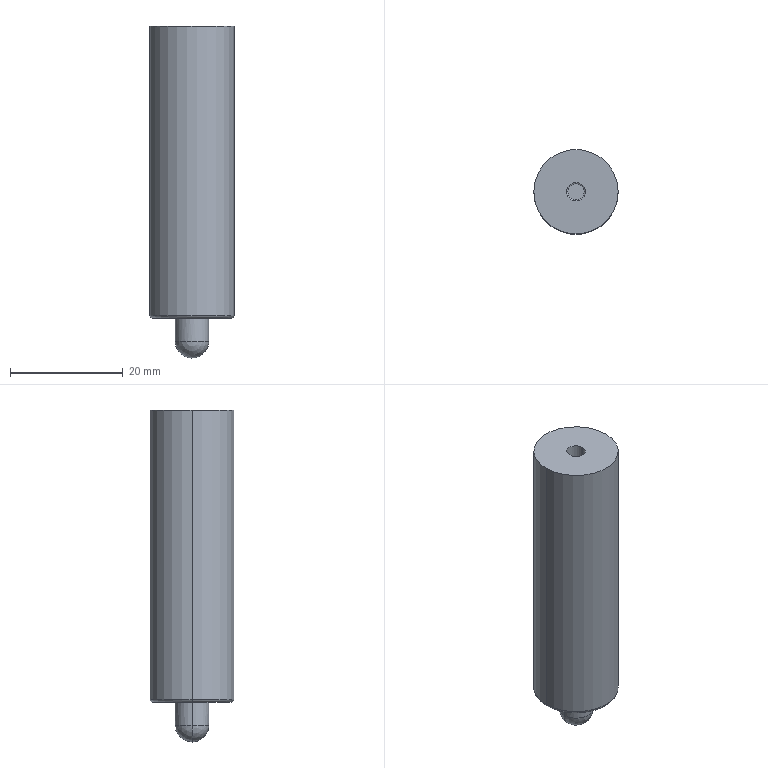Part | SolidWorks | features BaseBody 1, HoleWzd 1, MoveFace 1 | 1 solid | 18 faces | box 15 x 15 x 59 mm | volume 9190 mm3 | cylinder 8 | torus 3 | plane 3 | cone 2 | sphere 2 | commonest cylinder face diameters 2.9 x2 3.3 x2 6 x2 15 x2
STEP:
#1=CARTESIAN_POINT('',(-699.78,615.797,484.382));
#2=VERTEX_POINT('',#1);
#3=CARTESIAN_POINT('',(-696.48,615.797,484.382));
#4=VERTEX_POINT('',#3);
#5=CARTESIAN_POINT('',(-698.13,615.797,484.382));
#6=DIRECTION('',(0.,0.,1.));
#7=DIRECTION('',(1.,0.,0.));
#8=AXIS2_PLACEMENT_3D('',#5,#6,#7);
#9=CIRCLE('',#8,1.65);
#10=EDGE_CURVE('',#2,#4,#9,.T.);
#11=ORIENTED_EDGE('',*,*,#10,.F.);
#12=CARTESIAN_POINT('',(-699.78,615.797,494.482));
#13=VERTEX_POINT('',#12);
#14=CARTESIAN_POINT('',(-699.78,615.797,494.482));
#15=DIRECTION('',(0.,0.,1.));
#16=VECTOR('',#15,1000.);
#17=LINE('',#14,#16);
#18=EDGE_CURVE('',#2,#13,#17,.T.);
#19=ORIENTED_EDGE('',*,*,#18,.T.);
#20=CARTESIAN_POINT('',(-696.48,615.797,494.482));
#21=VERTEX_POINT('',#20);
#22=CARTESIAN_POINT('',(-698.13,615.797,494.482));
#23=DIRECTION('',(0.,0.,1.));
#24=DIRECTION('',(1.,0.,0.));
#25=AXIS2_PLACEMENT_3D('',#22,#23,#24);
#26=CIRCLE('',#25,1.65);
#27=EDGE_CURVE('',#13,#21,#26,.T.);
#28=ORIENTED_EDGE('',*,*,#27,.T.);
#29=CARTESIAN_POINT('',(-696.48,615.797,494.482));
#30=DIRECTION('',(0.,0.,1.));
#31=VECTOR('',#30,1000.);
#32=LINE('',#29,#31);
#33=EDGE_CURVE('',#4,#21,#32,.T.);
#34=ORIENTED_EDGE('',*,*,#33,.F.);
#35=EDGE_LOOP('',(#11,#19,#28,#34));
#36=FACE_OUTER_BOUND('',#35,.T.);
#37=CARTESIAN_POINT('',(-698.13,615.797,494.482));
#38=DIRECTION('',(0.,0.,1.));
#39=DIRECTION('',(1.,0.,0.));
#40=AXIS2_PLACEMENT_3D('',#37,#38,#39);
#41=CYLINDRICAL_SURFACE('',#40,1.65);
#42=ADVANCED_FACE('',(#36),#41,.F.);
#43=CARTESIAN_POINT('',(-699.58,615.797,484.262));
#44=VERTEX_POINT('',#43);
#45=CARTESIAN_POINT('',(-696.68,615.797,484.262));
#46=VERTEX_POINT('',#45);
#47=CARTESIAN_POINT('',(-698.13,615.797,484.262));
#48=DIRECTION('',(0.,0.,1.));
#49=DIRECTION('',(1.,0.,0.));
#50=AXIS2_PLACEMENT_3D('',#47,#48,#49);
#51=CIRCLE('',#50,1.45);
#52=EDGE_CURVE('',#44,#46,#51,.T.);
#53=ORIENTED_EDGE('',*,*,#52,.F.);
#54=CARTESIAN_POINT('',(-699.78,615.797,484.382));
#55=DIRECTION('',(-0.8572,0.,0.515));
#56=VECTOR('',#55,1000.);
#57=LINE('',#54,#56);
#58=EDGE_CURVE('',#44,#2,#57,.T.);
#59=ORIENTED_EDGE('',*,*,#58,.T.);
#60=ORIENTED_EDGE('',*,*,#10,.T.);
#61=CARTESIAN_POINT('',(-696.48,615.797,484.382));
#62=DIRECTION('',(0.8572,0.,0.515));
#63=VECTOR('',#62,1000.);
#64=LINE('',#61,#63);
#65=EDGE_CURVE('',#46,#4,#64,.T.);
#66=ORIENTED_EDGE('',*,*,#65,.F.);
#67=EDGE_LOOP('',(#53,#59,#60,#66));
#68=FACE_OUTER_BOUND('',#67,.T.);
#69=CARTESIAN_POINT('',(-698.13,615.797,484.382));
#70=DIRECTION('',(0.,0.,1.));
#71=DIRECTION('',(1.,0.,0.));
#72=AXIS2_PLACEMENT_3D('',#69,#70,#71);
#73=CONICAL_SURFACE('',#72,1.65,1.03);
#74=ADVANCED_FACE('',(#68),#73,.F.);
#75=CARTESIAN_POINT('',(-690.63,615.894,443.08));
#76=VERTEX_POINT('',#75);
#77=CARTESIAN_POINT('',(-705.63,615.797,443.08));
#78=VERTEX_POINT('',#77);
#79=CARTESIAN_POINT('',(-698.13,615.797,443.08));
#80=DIRECTION('',(0.,0.,1.));
#81=DIRECTION('',(0.9999,0.01286,0.));
#82=AXIS2_PLACEMENT_3D('',#79,#80,#81);
#83=CIRCLE('',#82,7.5);
#84=EDGE_CURVE('',#76,#78,#83,.T.);
#85=ORIENTED_EDGE('',*,*,#84,.F.);
#86=CARTESIAN_POINT('',(-691.13,615.887,442.58));
#87=VERTEX_POINT('',#86);
#88=CARTESIAN_POINT('',(-691.13,615.887,443.08));
#89=DIRECTION('',(-0.01286,0.9999,0.));
#90=DIRECTION('',(-0.9999,-0.01286,0.));
#91=AXIS2_PLACEMENT_3D('',#88,#89,#90);
#92=CIRCLE('',#91,0.5);
#93=EDGE_CURVE('',#76,#87,#92,.T.);
#94=ORIENTED_EDGE('',*,*,#93,.T.);
#95=CARTESIAN_POINT('',(-705.13,615.797,442.58));
#96=VERTEX_POINT('',#95);
#97=CARTESIAN_POINT('',(-698.13,615.797,442.58));
#98=DIRECTION('',(0.,0.,1.));
#99=DIRECTION('',(1.,0.000001544,0.));
#100=AXIS2_PLACEMENT_3D('',#97,#98,#99);
#101=CIRCLE('',#100,7.);
#102=EDGE_CURVE('',#87,#96,#101,.T.);
#103=ORIENTED_EDGE('',*,*,#102,.T.);
#104=CARTESIAN_POINT('',(-705.13,615.797,443.08));
#105=DIRECTION('',(0.000001544,-1.,0.));
#106=DIRECTION('',(-1.,-0.000001544,0.));
#107=AXIS2_PLACEMENT_3D('',#104,#105,#106);
#108=CIRCLE('',#107,0.5);
#109=EDGE_CURVE('',#78,#96,#108,.T.);
#110=ORIENTED_EDGE('',*,*,#109,.F.);
#111=EDGE_LOOP('',(#85,#94,#103,#110));
#112=FACE_OUTER_BOUND('',#111,.T.);
#113=CARTESIAN_POINT('',(-698.13,615.797,443.08));
#114=DIRECTION('',(0.,0.,-1.));
#115=DIRECTION('',(0.9999,0.01286,0.));
#116=AXIS2_PLACEMENT_3D('',#113,#114,#115);
#117=TOROIDAL_SURFACE('',#116,7.,0.5);
#118=ADVANCED_FACE('',(#112),#117,.T.);
#119=CARTESIAN_POINT('',(-698.13,615.797,494.482));
#120=DIRECTION('',(0.,0.,1.));
#121=DIRECTION('',(1.,0.,0.));
#122=AXIS2_PLACEMENT_3D('',#119,#120,#121);
#123=CIRCLE('',#122,1.65);
#124=EDGE_CURVE('',#21,#13,#123,.T.);
#125=ORIENTED_EDGE('',*,*,#124,.F.);
#126=ORIENTED_EDGE('',*,*,#27,.F.);
#127=EDGE_LOOP('',(#125,#126));
#128=FACE_BOUND('',#127,.T.);
#129=CARTESIAN_POINT('',(-705.63,615.797,494.482));
#130=VERTEX_POINT('',#129);
#131=CARTESIAN_POINT('',(-690.63,615.797,494.482));
#132=VERTEX_POINT('',#131);
#133=CARTESIAN_POINT('',(-698.13,615.797,494.482));
#134=DIRECTION('',(0.,0.,-1.));
#135=DIRECTION('',(-1.,-0.000001544,0.));
#136=AXIS2_PLACEMENT_3D('',#133,#134,#135);
#137=CIRCLE('',#136,7.5);
#138=EDGE_CURVE('',#130,#132,#137,.T.);
#139=ORIENTED_EDGE('',*,*,#138,.F.);
#140=CARTESIAN_POINT('',(-698.13,615.797,494.482));
#141=DIRECTION('',(0.,0.,-1.));
#142=DIRECTION('',(1.,0.000001544,0.));
#143=AXIS2_PLACEMENT_3D('',#140,#141,#142);
#144=CIRCLE('',#143,7.5);
#145=EDGE_CURVE('',#132,#130,#144,.T.);
#146=ORIENTED_EDGE('',*,*,#145,.F.);
#147=EDGE_LOOP('',(#139,#146));
#148=FACE_OUTER_BOUND('',#147,.T.);
#149=CARTESIAN_POINT('',(0.001745,0.001349,494.482));
#150=DIRECTION('',(0.,0.,-1.));
#151=DIRECTION('',(1.,0.000001544,0.));
#152=AXIS2_PLACEMENT_3D('',#149,#150,#151);
#153=PLANE('',#152);
#154=ADVANCED_FACE('',(#128,#148),#153,.F.);
#155=ORIENTED_EDGE('',*,*,#145,.T.);
#156=CARTESIAN_POINT('',(-705.63,615.797,494.482));
#157=DIRECTION('',(0.,0.,-1.));
#158=VECTOR('',#157,1000.);
#159=LINE('',#156,#158);
#160=EDGE_CURVE('',#130,#78,#159,.T.);
#161=ORIENTED_EDGE('',*,*,#160,.T.);
#162=CARTESIAN_POINT('',(-690.63,615.797,443.08));
#163=VERTEX_POINT('',#162);
#164=CARTESIAN_POINT('',(-698.13,615.797,443.08));
#165=DIRECTION('',(0.,0.,1.));
#166=DIRECTION('',(-1.,-0.000001544,0.));
#167=AXIS2_PLACEMENT_3D('',#164,#165,#166);
#168=CIRCLE('',#167,7.5);
#169=EDGE_CURVE('',#78,#163,#168,.T.);
#170=ORIENTED_EDGE('',*,*,#169,.T.);
#171=CARTESIAN_POINT('',(-690.63,615.797,443.08));
#172=DIRECTION('',(0.,0.,1.));
#173=VECTOR('',#172,1000.);
#174=LINE('',#171,#173);
#175=EDGE_CURVE('',#163,#132,#174,.T.);
#176=ORIENTED_EDGE('',*,*,#175,.T.);
#177=EDGE_LOOP('',(#155,#161,#170,#176));
#178=FACE_OUTER_BOUND('',#177,.T.);
#179=CARTESIAN_POINT('',(-698.13,615.797,442.58));
#180=DIRECTION('',(0.,0.,-1.));
#181=DIRECTION('',(1.,0.000001544,0.));
#182=AXIS2_PLACEMENT_3D('',#179,#180,#181);
#183=CYLINDRICAL_SURFACE('',#182,7.5);
#184=ADVANCED_FACE('',(#178),#183,.T.);
#185=ORIENTED_EDGE('',*,*,#138,.T.);
#186=ORIENTED_EDGE('',*,*,#175,.F.);
#187=CARTESIAN_POINT('',(-698.13,615.797,443.08));
#188=DIRECTION('',(0.,0.,1.));
#189=DIRECTION('',(0.9999,0.01286,0.));
#190=AXIS2_PLACEMENT_3D('',#187,#188,#189);
#191=CIRCLE('',#190,7.5);
#192=EDGE_CURVE('',#163,#76,#191,.T.);
#193=ORIENTED_EDGE('',*,*,#192,.T.);
#194=ORIENTED_EDGE('',*,*,#84,.T.);
#195=ORIENTED_EDGE('',*,*,#160,.F.);
#196=EDGE_LOOP('',(#185,#186,#193,#194,#195));
#197=FACE_OUTER_BOUND('',#196,.T.);
#198=CARTESIAN_POINT('',(-698.13,615.797,442.58));
#199=DIRECTION('',(0.,0.,-1.));
#200=DIRECTION('',(1.,0.000001544,0.));
#201=AXIS2_PLACEMENT_3D('',#198,#199,#200);
#202=CYLINDRICAL_SURFACE('',#201,7.5);
#203=ADVANCED_FACE('',(#197),#202,.T.);
#204=ORIENTED_EDGE('',*,*,#93,.F.);
#205=ORIENTED_EDGE('',*,*,#192,.F.);
#206=CARTESIAN_POINT('',(-691.13,615.797,442.58));
#207=VERTEX_POINT('',#206);
#208=CARTESIAN_POINT('',(-691.13,615.797,443.08));
#209=DIRECTION('',(0.000001544,-1.,0.));
#210=DIRECTION('',(0.,0.,-1.));
#211=AXIS2_PLACEMENT_3D('',#208,#209,#210);
#212=CIRCLE('',#211,0.5);
#213=EDGE_CURVE('',#207,#163,#212,.T.);
#214=ORIENTED_EDGE('',*,*,#213,.F.);
#215=CARTESIAN_POINT('',(-698.13,615.797,442.58));
#216=DIRECTION('',(0.,0.,1.));
#217=DIRECTION('',(1.,0.000001544,0.));
#218=AXIS2_PLACEMENT_3D('',#215,#216,#217);
#219=CIRCLE('',#218,7.);
#220=EDGE_CURVE('',#207,#87,#219,.T.);
#221=ORIENTED_EDGE('',*,*,#220,.T.);
#222=EDGE_LOOP('',(#204,#205,#214,#221));
#223=FACE_OUTER_BOUND('',#222,.T.);
#224=CARTESIAN_POINT('',(-698.13,615.797,443.08));
#225=DIRECTION('',(0.,0.,-1.));
#226=DIRECTION('',(0.9999,0.01286,0.));
#227=AXIS2_PLACEMENT_3D('',#224,#225,#226);
#228=TOROIDAL_SURFACE('',#227,7.,0.5);
#229=ADVANCED_FACE('',(#223),#228,.T.);
#230=ORIENTED_EDGE('',*,*,#169,.F.);
#231=ORIENTED_EDGE('',*,*,#109,.T.);
#232=CARTESIAN_POINT('',(-698.13,615.797,442.58));
#233=DIRECTION('',(0.,0.,1.));
#234=DIRECTION('',(-1.,-0.000001544,0.));
#235=AXIS2_PLACEMENT_3D('',#232,#233,#234);
#236=CIRCLE('',#235,7.);
#237=EDGE_CURVE('',#96,#207,#236,.T.);
#238=ORIENTED_EDGE('',*,*,#237,.T.);
#239=ORIENTED_EDGE('',*,*,#213,.T.);
#240=EDGE_LOOP('',(#230,#231,#238,#239));
#241=FACE_OUTER_BOUND('',#240,.T.);
#242=CARTESIAN_POINT('',(-698.13,615.797,443.08));
#243=DIRECTION('',(0.,0.,-1.));
#244=DIRECTION('',(1.,0.000001544,0.));
#245=AXIS2_PLACEMENT_3D('',#242,#243,#244);
#246=TOROIDAL_SURFACE('',#245,7.,0.5);
#247=ADVANCED_FACE('',(#241),#246,.T.);
#248=ORIENTED_EDGE('',*,*,#237,.F.);
#249=ORIENTED_EDGE('',*,*,#102,.F.);
#250=ORIENTED_EDGE('',*,*,#220,.F.);
#251=EDGE_LOOP('',(#248,#249,#250));
#252=FACE_OUTER_BOUND('',#251,.T.);
#253=CARTESIAN_POINT('',(-695.13,615.797,442.58));
#254=VERTEX_POINT('',#253);
#255=CARTESIAN_POINT('',(-701.13,615.797,442.58));
#256=VERTEX_POINT('',#255);
#257=CARTESIAN_POINT('',(-698.13,615.797,442.58));
#258=DIRECTION('',(0.,0.,-1.));
#259=DIRECTION('',(1.,0.000001544,0.));
#260=AXIS2_PLACEMENT_3D('',#257,#258,#259);
#261=CIRCLE('',#260,3.);
#262=EDGE_CURVE('',#254,#256,#261,.T.);
#263=ORIENTED_EDGE('',*,*,#262,.F.);
#264=CARTESIAN_POINT('',(-698.13,615.797,442.58));
#265=DIRECTION('',(0.,0.,-1.));
#266=DIRECTION('',(-1.,-0.000001544,0.));
#267=AXIS2_PLACEMENT_3D('',#264,#265,#266);
#268=CIRCLE('',#267,3.);
#269=EDGE_CURVE('',#256,#254,#268,.T.);
#270=ORIENTED_EDGE('',*,*,#269,.F.);
#271=EDGE_LOOP('',(#263,#270));
#272=FACE_BOUND('',#271,.T.);
#273=CARTESIAN_POINT('',(-653.13,626.297,442.58));
#274=DIRECTION('',(0.,0.,1.));
#275=DIRECTION('',(-0.000001544,1.,0.));
#276=AXIS2_PLACEMENT_3D('',#273,#274,#275);
#277=PLANE('',#276);
#278=ADVANCED_FACE('',(#252,#272),#277,.F.);
#279=ORIENTED_EDGE('',*,*,#269,.T.);
#280=CARTESIAN_POINT('',(-695.13,615.797,438.482));
#281=VERTEX_POINT('',#280);
#282=CARTESIAN_POINT('',(-695.13,615.797,442.58));
#283=DIRECTION('',(0.,0.,-1.));
#284=VECTOR('',#283,1000.);
#285=LINE('',#282,#284);
#286=EDGE_CURVE('',#254,#281,#285,.T.);
#287=ORIENTED_EDGE('',*,*,#286,.T.);
#288=CARTESIAN_POINT('',(-701.13,615.797,438.482));
#289=VERTEX_POINT('',#288);
#290=CARTESIAN_POINT('',(-698.13,615.797,438.482));
#291=DIRECTION('',(0.,0.,1.));
#292=DIRECTION('',(1.,0.000001544,0.));
#293=AXIS2_PLACEMENT_3D('',#290,#291,#292);
#294=CIRCLE('',#293,3.);
#295=EDGE_CURVE('',#281,#289,#294,.T.);
#296=ORIENTED_EDGE('',*,*,#295,.T.);
#297=CARTESIAN_POINT('',(-701.13,615.797,438.482));
#298=DIRECTION('',(0.,0.,1.));
#299=VECTOR('',#298,1000.);
#300=LINE('',#297,#299);
#301=EDGE_CURVE('',#289,#256,#300,.T.);
#302=ORIENTED_EDGE('',*,*,#301,.T.);
#303=EDGE_LOOP('',(#279,#287,#296,#302));
#304=FACE_OUTER_BOUND('',#303,.T.);
#305=CARTESIAN_POINT('',(-698.13,615.797,442.58));
#306=DIRECTION('',(0.,0.,-1.));
#307=DIRECTION('',(1.,0.000001544,0.));
#308=AXIS2_PLACEMENT_3D('',#305,#306,#307);
#309=CYLINDRICAL_SURFACE('',#308,3.);
#310=ADVANCED_FACE('',(#304),#309,.T.);
#311=ORIENTED_EDGE('',*,*,#262,.T.);
#312=ORIENTED_EDGE('',*,*,#301,.F.);
#313=CARTESIAN_POINT('',(-698.13,615.797,438.482));
#314=DIRECTION('',(0.,0.,1.));
#315=DIRECTION('',(-1.,-0.000001544,0.));
#316=AXIS2_PLACEMENT_3D('',#313,#314,#315);
#317=CIRCLE('',#316,3.);
#318=EDGE_CURVE('',#289,#281,#317,.T.);
#319=ORIENTED_EDGE('',*,*,#318,.T.);
#320=ORIENTED_EDGE('',*,*,#286,.F.);
#321=EDGE_LOOP('',(#311,#312,#319,#320));
#322=FACE_OUTER_BOUND('',#321,.T.);
#323=CARTESIAN_POINT('',(-698.13,615.797,442.58));
#324=DIRECTION('',(0.,0.,-1.));
#325=DIRECTION('',(1.,0.000001544,0.));
#326=AXIS2_PLACEMENT_3D('',#323,#324,#325);
#327=CYLINDRICAL_SURFACE('',#326,3.);
#328=ADVANCED_FACE('',(#322),#327,.T.);
#329=CARTESIAN_POINT('',(-698.13,615.797,435.482));
#330=VERTEX_POINT('',#329);
#331=CARTESIAN_POINT('',(-698.13,615.797,438.482));
#332=DIRECTION('',(-0.000001545,1.,0.));
#333=DIRECTION('',(1.,0.000001545,0.));
#334=AXIS2_PLACEMENT_3D('',#331,#332,#333);
#335=CIRCLE('',#334,3.);
#336=EDGE_CURVE('',#281,#330,#335,.T.);
#337=ORIENTED_EDGE('',*,*,#336,.F.);
#338=ORIENTED_EDGE('',*,*,#318,.F.);
#339=CARTESIAN_POINT('',(-698.13,615.797,438.482));
#340=DIRECTION('',(-0.000001544,1.,0.));
#341=DIRECTION('',(0.,0.,-1.));
#342=AXIS2_PLACEMENT_3D('',#339,#340,#341);
#343=CIRCLE('',#342,3.);
#344=EDGE_CURVE('',#330,#289,#343,.T.);
#345=ORIENTED_EDGE('',*,*,#344,.F.);
#346=EDGE_LOOP('',(#337,#338,#345));
#347=FACE_OUTER_BOUND('',#346,.T.);
#348=CARTESIAN_POINT('',(-698.13,615.797,438.482));
#349=DIRECTION('',(0.000001544,-1.,0.));
#350=DIRECTION('',(1.,0.000001544,0.));
#351=AXIS2_PLACEMENT_3D('',#348,#349,#350);
#352=SPHERICAL_SURFACE('',#351,3.);
#353=ADVANCED_FACE('',(#347),#352,.T.);
#354=ORIENTED_EDGE('',*,*,#344,.T.);
#355=ORIENTED_EDGE('',*,*,#295,.F.);
#356=ORIENTED_EDGE('',*,*,#336,.T.);
#357=EDGE_LOOP('',(#354,#355,#356));
#358=FACE_OUTER_BOUND('',#357,.T.);
#359=CARTESIAN_POINT('',(-698.13,615.797,438.482));
#360=DIRECTION('',(0.000001544,-1.,0.));
#361=DIRECTION('',(1.,0.000001544,0.));
#362=AXIS2_PLACEMENT_3D('',#359,#360,#361);
#363=SPHERICAL_SURFACE('',#362,3.);
#364=ADVANCED_FACE('',(#358),#363,.T.);
#365=ORIENTED_EDGE('',*,*,#58,.F.);
#366=CARTESIAN_POINT('',(-698.13,615.797,484.262));
#367=DIRECTION('',(0.,0.,1.));
#368=DIRECTION('',(1.,0.,0.));
#369=AXIS2_PLACEMENT_3D('',#366,#367,#368);
#370=CIRCLE('',#369,1.45);
#371=EDGE_CURVE('',#46,#44,#370,.T.);
#372=ORIENTED_EDGE('',*,*,#371,.F.);
#373=ORIENTED_EDGE('',*,*,#65,.T.);
#374=CARTESIAN_POINT('',(-698.13,615.797,484.382));
#375=DIRECTION('',(0.,0.,1.));
#376=DIRECTION('',(1.,0.,0.));
#377=AXIS2_PLACEMENT_3D('',#374,#375,#376);
#378=CIRCLE('',#377,1.65);
#379=EDGE_CURVE('',#4,#2,#378,.T.);
#380=ORIENTED_EDGE('',*,*,#379,.T.);
#381=EDGE_LOOP('',(#365,#372,#373,#380));
#382=FACE_OUTER_BOUND('',#381,.T.);
#383=CARTESIAN_POINT('',(-698.13,615.797,484.382));
#384=DIRECTION('',(0.,0.,1.));
#385=DIRECTION('',(1.,0.,0.));
#386=AXIS2_PLACEMENT_3D('',#383,#384,#385);
#387=CONICAL_SURFACE('',#386,1.65,1.03);
#388=ADVANCED_FACE('',(#382),#387,.F.);
#389=ORIENTED_EDGE('',*,*,#18,.F.);
#390=ORIENTED_EDGE('',*,*,#379,.F.);
#391=ORIENTED_EDGE('',*,*,#33,.T.);
#392=ORIENTED_EDGE('',*,*,#124,.T.);
#393=EDGE_LOOP('',(#389,#390,#391,#392));
#394=FACE_OUTER_BOUND('',#393,.T.);
#395=CARTESIAN_POINT('',(-698.13,615.797,494.482));
#396=DIRECTION('',(0.,0.,1.));
#397=DIRECTION('',(1.,0.,0.));
#398=AXIS2_PLACEMENT_3D('',#395,#396,#397);
#399=CYLINDRICAL_SURFACE('',#398,1.65);
#400=ADVANCED_FACE('',(#394),#399,.F.);
#401=CARTESIAN_POINT('',(-699.58,615.797,474.482));
#402=VERTEX_POINT('',#401);
#403=CARTESIAN_POINT('',(-696.68,615.797,474.482));
#404=VERTEX_POINT('',#403);
#405=CARTESIAN_POINT('',(-698.13,615.797,474.482));
#406=DIRECTION('',(0.,0.,-1.));
#407=DIRECTION('',(1.,0.,0.));
#408=AXIS2_PLACEMENT_3D('',#405,#406,#407);
#409=CIRCLE('',#408,1.45);
#410=EDGE_CURVE('',#402,#404,#409,.T.);
#411=ORIENTED_EDGE('',*,*,#410,.F.);
#412=CARTESIAN_POINT('',(-698.13,615.797,474.482));
#413=DIRECTION('',(0.,0.,-1.));
#414=DIRECTION('',(1.,0.,0.));
#415=AXIS2_PLACEMENT_3D('',#412,#413,#414);
#416=CIRCLE('',#415,1.45);
#417=EDGE_CURVE('',#404,#402,#416,.T.);
#418=ORIENTED_EDGE('',*,*,#417,.F.);
#419=EDGE_LOOP('',(#411,#418));
#420=FACE_OUTER_BOUND('',#419,.T.);
#421=CARTESIAN_POINT('',(0.001745,0.001349,474.482));
#422=DIRECTION('',(0.,0.,1.));
#423=DIRECTION('',(-1.,-0.000001544,0.));
#424=AXIS2_PLACEMENT_3D('',#421,#422,#423);
#425=PLANE('',#424);
#426=ADVANCED_FACE('',(#420),#425,.T.);
#427=CARTESIAN_POINT('',(-696.68,615.797,494.482));
#428=DIRECTION('',(0.,0.,-1.));
#429=VECTOR('',#428,1000.);
#430=LINE('',#427,#429);
#431=EDGE_CURVE('',#46,#404,#430,.T.);
#432=ORIENTED_EDGE('',*,*,#431,.F.);
#433=ORIENTED_EDGE('',*,*,#371,.T.);
#434=CARTESIAN_POINT('',(-699.58,615.797,494.482));
#435=DIRECTION('',(0.,0.,1.));
#436=VECTOR('',#435,1000.);
#437=LINE('',#434,#436);
#438=EDGE_CURVE('',#402,#44,#437,.T.);
#439=ORIENTED_EDGE('',*,*,#438,.F.);
#440=ORIENTED_EDGE('',*,*,#410,.T.);
#441=EDGE_LOOP('',(#432,#433,#439,#440));
#442=FACE_OUTER_BOUND('',#441,.T.);
#443=CARTESIAN_POINT('',(-698.13,615.797,494.482));
#444=DIRECTION('',(0.,0.,1.));
#445=DIRECTION('',(-1.,-0.000001544,0.));
#446=AXIS2_PLACEMENT_3D('',#443,#444,#445);
#447=CYLINDRICAL_SURFACE('',#446,1.45);
#448=ADVANCED_FACE('',(#442),#447,.F.);
#449=ORIENTED_EDGE('',*,*,#438,.T.);
#450=ORIENTED_EDGE('',*,*,#52,.T.);
#451=ORIENTED_EDGE('',*,*,#431,.T.);
#452=ORIENTED_EDGE('',*,*,#417,.T.);
#453=EDGE_LOOP('',(#449,#450,#451,#452));
#454=FACE_OUTER_BOUND('',#453,.T.);
#455=CARTESIAN_POINT('',(-698.13,615.797,494.482));
#456=DIRECTION('',(0.,0.,1.));
#457=DIRECTION('',(-1.,-0.000001544,0.));
#458=AXIS2_PLACEMENT_3D('',#455,#456,#457);
#459=CYLINDRICAL_SURFACE('',#458,1.45);
#460=ADVANCED_FACE('',(#454),#459,.F.);
#461=CLOSED_SHELL('',(#42,#74,#118,#154,#184,#203,#229,#247,#278,#310,#328,#353,#364,#388,#400,#426,#448,#460));
#462=MANIFOLD_SOLID_BREP('',#461);
#463=CARTESIAN_POINT('',(0.,0.,0.));
#464=DIRECTION('',(0.,0.,1.));
#465=DIRECTION('',(1.,0.,0.));
#466=AXIS2_PLACEMENT_3D('',#463,#464,#465);
#467=(LENGTH_UNIT()NAMED_UNIT(*)SI_UNIT(.MILLI.,.METRE.));
#468=UNCERTAINTY_MEASURE_WITH_UNIT(LENGTH_MEASURE(0.00001),#467,'','');
#469=(NAMED_UNIT(*)PLANE_ANGLE_UNIT()SI_UNIT($,.RADIAN.));
#470=(NAMED_UNIT(*)SI_UNIT($,.STERADIAN.)SOLID_ANGLE_UNIT());
#471=(GEOMETRIC_REPRESENTATION_CONTEXT(3)GLOBAL_UNCERTAINTY_ASSIGNED_CONTEXT((#468))GLOBAL_UNIT_ASSIGNED_CONTEXT((#467,#469,#470))REPRESENTATION_CONTEXT('',''));
#472=ADVANCED_BREP_SHAPE_REPRESENTATION('',(#462,#466),#471);